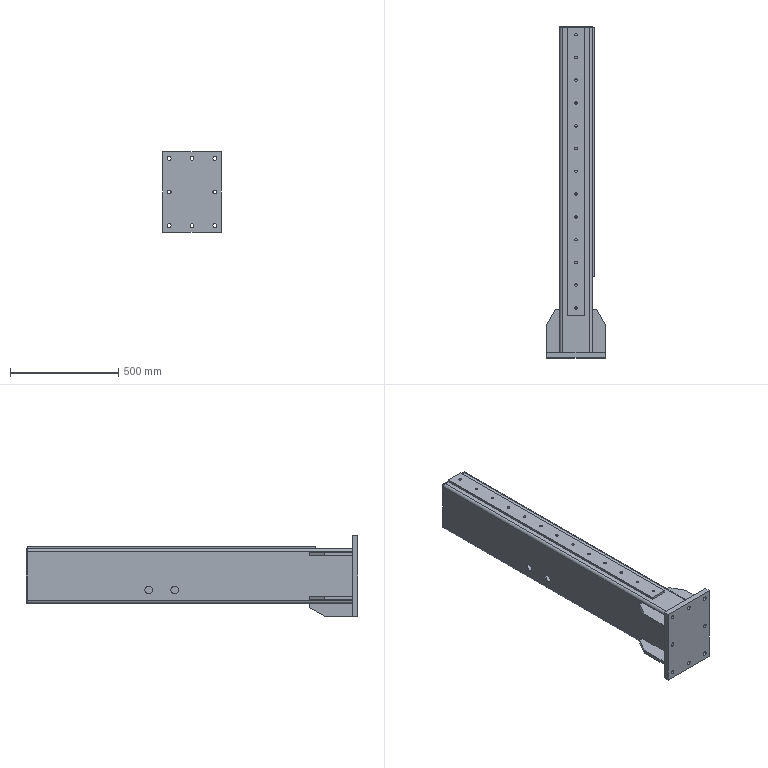Part | SolidWorks | features ICE 8, HoleWzd 3, MirrorSolid 2, WeldMemberFeat 1, WeldmentFeature 1 | 11 solids | 185 faces | box 270 x 1530 x 370 mm | volume 12311582 mm3 | cylinder 96 | plane 89 | commonest cylinder face diameters 12 x52 17.5 x24 25.2 x8 12.6 x4 15.5 x4 35 x4